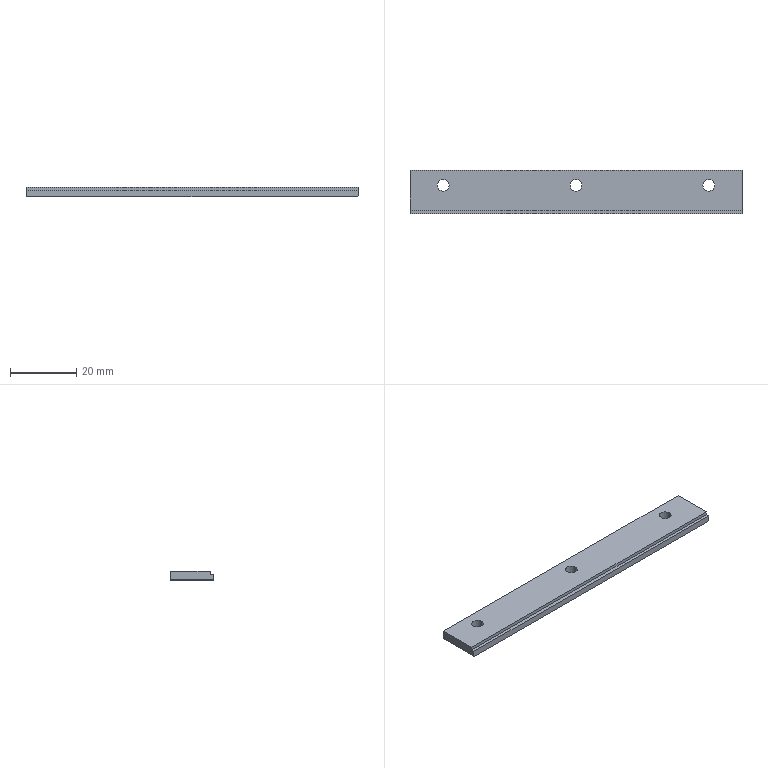Part | STEP file | Feed slide cover_Default | 1 solid | 16 faces | box 100 x 13 x 3 mm | volume 3712 mm3 | plane 10 | cylinder 6 | commonest cylinder face diameters 3.5 x6
STEP:
#1=CARTESIAN_POINT('',(0.,0.,0.));
#2=DIRECTION('',(0.,0.,1.));
#3=DIRECTION('',(1.,0.,0.));
#4=AXIS2_PLACEMENT_3D('',#1,#2,#3);
#5=CARTESIAN_POINT('',(12.886,5.77,0.));
#6=VERTEX_POINT('',#5);
#7=CARTESIAN_POINT('',(12.886,5.77,3.));
#8=VERTEX_POINT('',#7);
#9=CARTESIAN_POINT('',(12.886,5.77,0.));
#10=DIRECTION('',(0.,0.,1.));
#11=VECTOR('',#10,1.);
#12=LINE('',#9,#11);
#13=CARTESIAN_POINT('',(11.136,5.77,0.));
#14=DIRECTION('',(0.,0.,1.));
#15=DIRECTION('',(1.,0.,0.));
#16=AXIS2_PLACEMENT_3D('',#13,#14,#15);
#17=CYLINDRICAL_SURFACE('',#16,1.75);
#18=CARTESIAN_POINT('',(6.283,0.));
#19=DIRECTION('',(0.,1.));
#20=VECTOR('',#19,1.);
#21=LINE('',#18,#20);
#22=(GEOMETRIC_REPRESENTATION_CONTEXT(2)PARAMETRIC_REPRESENTATION_CONTEXT()REPRESENTATION_CONTEXT('',''));
#23=DEFINITIONAL_REPRESENTATION('',(#21),#22);
#24=PCURVE('',#17,#23);
#25=CARTESIAN_POINT('',(11.136,5.77,0.));
#26=DIRECTION('',(0.,0.,1.));
#27=DIRECTION('',(1.,0.,0.));
#28=AXIS2_PLACEMENT_3D('',#25,#26,#27);
#29=CYLINDRICAL_SURFACE('',#28,1.75);
#30=CARTESIAN_POINT('',(0.,0.));
#31=DIRECTION('',(0.,1.));
#32=VECTOR('',#31,1.);
#33=LINE('',#30,#32);
#34=(GEOMETRIC_REPRESENTATION_CONTEXT(2)PARAMETRIC_REPRESENTATION_CONTEXT()REPRESENTATION_CONTEXT('',''));
#35=DEFINITIONAL_REPRESENTATION('',(#33),#34);
#36=PCURVE('',#29,#35);
#37=SURFACE_CURVE('',#12,(#24,#36),.PCURVE_S1.);
#38=EDGE_CURVE('',#6,#8,#37,.T.);
#39=ORIENTED_EDGE('',*,*,#38,.T.);
#40=CARTESIAN_POINT('',(9.386,5.77,3.));
#41=VERTEX_POINT('',#40);
#42=CARTESIAN_POINT('',(11.136,5.77,3.));
#43=DIRECTION('',(0.,0.,1.));
#44=DIRECTION('',(1.,0.,0.));
#45=AXIS2_PLACEMENT_3D('',#42,#43,#44);
#46=CIRCLE('',#45,1.75);
#47=CARTESIAN_POINT('',(0.,3.));
#48=DIRECTION('',(1.,0.));
#49=VECTOR('',#48,1.);
#50=LINE('',#47,#49);
#51=(GEOMETRIC_REPRESENTATION_CONTEXT(2)PARAMETRIC_REPRESENTATION_CONTEXT()REPRESENTATION_CONTEXT('',''));
#52=DEFINITIONAL_REPRESENTATION('',(#50),#51);
#53=PCURVE('',#17,#52);
#54=CARTESIAN_POINT('',(1.136,10.27,3.));
#55=DIRECTION('',(0.,0.,-1.));
#56=DIRECTION('',(-1.,0.,0.));
#57=AXIS2_PLACEMENT_3D('',#54,#55,#56);
#58=PLANE('',#57);
#59=CARTESIAN_POINT('',(-11.75,-4.5));
#60=CARTESIAN_POINT('',(-11.75,-1.469));
#61=CARTESIAN_POINT('',(-9.125,-2.984));
#62=CARTESIAN_POINT('',(-6.5,-4.5));
#63=CARTESIAN_POINT('',(-9.125,-6.016));
#64=CARTESIAN_POINT('',(-11.75,-7.531));
#65=CARTESIAN_POINT('',(-11.75,-4.5));
#66=(BOUNDED_CURVE()B_SPLINE_CURVE(2,(#59,#60,#61,#62,#63,#64,#65),.UNSPECIFIED.,.T.,.F.)B_SPLINE_CURVE_WITH_KNOTS((1,2,2,2,2,1),(-2.094,0.,2.094,4.189,6.283,8.378),.UNSPECIFIED.)CURVE()GEOMETRIC_REPRESENTATION_ITEM()RATIONAL_B_SPLINE_CURVE((1.,0.5,1.,0.5,1.,0.5,1.))REPRESENTATION_ITEM(''));
#67=(GEOMETRIC_REPRESENTATION_CONTEXT(2)PARAMETRIC_REPRESENTATION_CONTEXT()REPRESENTATION_CONTEXT('',''));
#68=DEFINITIONAL_REPRESENTATION('',(#66),#67);
#69=PCURVE('',#58,#68);
#70=SURFACE_CURVE('',#46,(#53,#69),.PCURVE_S1.);
#71=EDGE_CURVE('',#41,#8,#70,.T.);
#72=ORIENTED_EDGE('',*,*,#71,.F.);
#73=CARTESIAN_POINT('',(9.386,5.77,0.));
#74=VERTEX_POINT('',#73);
#75=CARTESIAN_POINT('',(9.386,5.77,0.));
#76=DIRECTION('',(0.,0.,1.));
#77=VECTOR('',#76,1.);
#78=LINE('',#75,#77);
#79=CARTESIAN_POINT('',(3.142,0.));
#80=DIRECTION('',(0.,1.));
#81=VECTOR('',#80,1.);
#82=LINE('',#79,#81);
#83=(GEOMETRIC_REPRESENTATION_CONTEXT(2)PARAMETRIC_REPRESENTATION_CONTEXT()REPRESENTATION_CONTEXT('',''));
#84=DEFINITIONAL_REPRESENTATION('',(#82),#83);
#85=PCURVE('',#17,#84);
#86=CARTESIAN_POINT('',(3.142,0.));
#87=DIRECTION('',(0.,1.));
#88=VECTOR('',#87,1.);
#89=LINE('',#86,#88);
#90=(GEOMETRIC_REPRESENTATION_CONTEXT(2)PARAMETRIC_REPRESENTATION_CONTEXT()REPRESENTATION_CONTEXT('',''));
#91=DEFINITIONAL_REPRESENTATION('',(#89),#90);
#92=PCURVE('',#29,#91);
#93=SURFACE_CURVE('',#78,(#85,#92),.PCURVE_S1.);
#94=EDGE_CURVE('',#74,#41,#93,.T.);
#95=ORIENTED_EDGE('',*,*,#94,.F.);
#96=CARTESIAN_POINT('',(11.136,5.77,0.));
#97=DIRECTION('',(0.,0.,1.));
#98=DIRECTION('',(1.,0.,0.));
#99=AXIS2_PLACEMENT_3D('',#96,#97,#98);
#100=CIRCLE('',#99,1.75);
#101=CARTESIAN_POINT('',(0.,0.));
#102=DIRECTION('',(1.,0.));
#103=VECTOR('',#102,1.);
#104=LINE('',#101,#103);
#105=(GEOMETRIC_REPRESENTATION_CONTEXT(2)PARAMETRIC_REPRESENTATION_CONTEXT()REPRESENTATION_CONTEXT('',''));
#106=DEFINITIONAL_REPRESENTATION('',(#104),#105);
#107=PCURVE('',#17,#106);
#108=CARTESIAN_POINT('',(1.136,10.27,0.));
#109=DIRECTION('',(0.,0.,-1.));
#110=DIRECTION('',(-1.,0.,0.));
#111=AXIS2_PLACEMENT_3D('',#108,#109,#110);
#112=PLANE('',#111);
#113=CARTESIAN_POINT('',(-11.75,-4.5));
#114=CARTESIAN_POINT('',(-11.75,-1.469));
#115=CARTESIAN_POINT('',(-9.125,-2.984));
#116=CARTESIAN_POINT('',(-6.5,-4.5));
#117=CARTESIAN_POINT('',(-9.125,-6.016));
#118=CARTESIAN_POINT('',(-11.75,-7.531));
#119=CARTESIAN_POINT('',(-11.75,-4.5));
#120=(BOUNDED_CURVE()B_SPLINE_CURVE(2,(#113,#114,#115,#116,#117,#118,#119),.UNSPECIFIED.,.T.,.F.)B_SPLINE_CURVE_WITH_KNOTS((1,2,2,2,2,1),(-2.094,0.,2.094,4.189,6.283,8.378),.UNSPECIFIED.)CURVE()GEOMETRIC_REPRESENTATION_ITEM()RATIONAL_B_SPLINE_CURVE((1.,0.5,1.,0.5,1.,0.5,1.))REPRESENTATION_ITEM(''));
#121=(GEOMETRIC_REPRESENTATION_CONTEXT(2)PARAMETRIC_REPRESENTATION_CONTEXT()REPRESENTATION_CONTEXT('',''));
#122=DEFINITIONAL_REPRESENTATION('',(#120),#121);
#123=PCURVE('',#112,#122);
#124=SURFACE_CURVE('',#100,(#107,#123),.PCURVE_S1.);
#125=EDGE_CURVE('',#74,#6,#124,.T.);
#126=ORIENTED_EDGE('',*,*,#125,.T.);
#127=EDGE_LOOP('',(#39,#72,#95,#126));
#128=FACE_BOUND('',#127,.F.);
#129=ADVANCED_FACE('',(#128),#17,.F.);
#130=CARTESIAN_POINT('',(52.886,5.77,0.));
#131=VERTEX_POINT('',#130);
#132=CARTESIAN_POINT('',(52.886,5.77,3.));
#133=VERTEX_POINT('',#132);
#134=CARTESIAN_POINT('',(52.886,5.77,0.));
#135=DIRECTION('',(0.,0.,1.));
#136=VECTOR('',#135,1.);
#137=LINE('',#134,#136);
#138=CARTESIAN_POINT('',(51.136,5.77,0.));
#139=DIRECTION('',(0.,0.,1.));
#140=DIRECTION('',(1.,0.,0.));
#141=AXIS2_PLACEMENT_3D('',#138,#139,#140);
#142=CYLINDRICAL_SURFACE('',#141,1.75);
#143=CARTESIAN_POINT('',(6.283,0.));
#144=DIRECTION('',(0.,1.));
#145=VECTOR('',#144,1.);
#146=LINE('',#143,#145);
#147=(GEOMETRIC_REPRESENTATION_CONTEXT(2)PARAMETRIC_REPRESENTATION_CONTEXT()REPRESENTATION_CONTEXT('',''));
#148=DEFINITIONAL_REPRESENTATION('',(#146),#147);
#149=PCURVE('',#142,#148);
#150=CARTESIAN_POINT('',(51.136,5.77,0.));
#151=DIRECTION('',(0.,0.,1.));
#152=DIRECTION('',(1.,0.,0.));
#153=AXIS2_PLACEMENT_3D('',#150,#151,#152);
#154=CYLINDRICAL_SURFACE('',#153,1.75);
#155=CARTESIAN_POINT('',(0.,0.));
#156=DIRECTION('',(0.,1.));
#157=VECTOR('',#156,1.);
#158=LINE('',#155,#157);
#159=(GEOMETRIC_REPRESENTATION_CONTEXT(2)PARAMETRIC_REPRESENTATION_CONTEXT()REPRESENTATION_CONTEXT('',''));
#160=DEFINITIONAL_REPRESENTATION('',(#158),#159);
#161=PCURVE('',#154,#160);
#162=SURFACE_CURVE('',#137,(#149,#161),.PCURVE_S1.);
#163=EDGE_CURVE('',#131,#133,#162,.T.);
#164=ORIENTED_EDGE('',*,*,#163,.T.);
#165=CARTESIAN_POINT('',(49.386,5.77,3.));
#166=VERTEX_POINT('',#165);
#167=CARTESIAN_POINT('',(51.136,5.77,3.));
#168=DIRECTION('',(0.,0.,1.));
#169=DIRECTION('',(1.,0.,0.));
#170=AXIS2_PLACEMENT_3D('',#167,#168,#169);
#171=CIRCLE('',#170,1.75);
#172=CARTESIAN_POINT('',(0.,3.));
#173=DIRECTION('',(1.,0.));
#174=VECTOR('',#173,1.);
#175=LINE('',#172,#174);
#176=(GEOMETRIC_REPRESENTATION_CONTEXT(2)PARAMETRIC_REPRESENTATION_CONTEXT()REPRESENTATION_CONTEXT('',''));
#177=DEFINITIONAL_REPRESENTATION('',(#175),#176);
#178=PCURVE('',#142,#177);
#179=CARTESIAN_POINT('',(-51.75,-4.5));
#180=CARTESIAN_POINT('',(-51.75,-1.469));
#181=CARTESIAN_POINT('',(-49.125,-2.984));
#182=CARTESIAN_POINT('',(-46.5,-4.5));
#183=CARTESIAN_POINT('',(-49.125,-6.016));
#184=CARTESIAN_POINT('',(-51.75,-7.531));
#185=CARTESIAN_POINT('',(-51.75,-4.5));
#186=(BOUNDED_CURVE()B_SPLINE_CURVE(2,(#179,#180,#181,#182,#183,#184,#185),.UNSPECIFIED.,.T.,.F.)B_SPLINE_CURVE_WITH_KNOTS((1,2,2,2,2,1),(-2.094,0.,2.094,4.189,6.283,8.378),.UNSPECIFIED.)CURVE()GEOMETRIC_REPRESENTATION_ITEM()RATIONAL_B_SPLINE_CURVE((1.,0.5,1.,0.5,1.,0.5,1.))REPRESENTATION_ITEM(''));
#187=(GEOMETRIC_REPRESENTATION_CONTEXT(2)PARAMETRIC_REPRESENTATION_CONTEXT()REPRESENTATION_CONTEXT('',''));
#188=DEFINITIONAL_REPRESENTATION('',(#186),#187);
#189=PCURVE('',#58,#188);
#190=SURFACE_CURVE('',#171,(#178,#189),.PCURVE_S1.);
#191=EDGE_CURVE('',#166,#133,#190,.T.);
#192=ORIENTED_EDGE('',*,*,#191,.F.);
#193=CARTESIAN_POINT('',(49.386,5.77,0.));
#194=VERTEX_POINT('',#193);
#195=CARTESIAN_POINT('',(49.386,5.77,0.));
#196=DIRECTION('',(0.,0.,1.));
#197=VECTOR('',#196,1.);
#198=LINE('',#195,#197);
#199=CARTESIAN_POINT('',(3.142,0.));
#200=DIRECTION('',(0.,1.));
#201=VECTOR('',#200,1.);
#202=LINE('',#199,#201);
#203=(GEOMETRIC_REPRESENTATION_CONTEXT(2)PARAMETRIC_REPRESENTATION_CONTEXT()REPRESENTATION_CONTEXT('',''));
#204=DEFINITIONAL_REPRESENTATION('',(#202),#203);
#205=PCURVE('',#142,#204);
#206=CARTESIAN_POINT('',(3.142,0.));
#207=DIRECTION('',(0.,1.));
#208=VECTOR('',#207,1.);
#209=LINE('',#206,#208);
#210=(GEOMETRIC_REPRESENTATION_CONTEXT(2)PARAMETRIC_REPRESENTATION_CONTEXT()REPRESENTATION_CONTEXT('',''));
#211=DEFINITIONAL_REPRESENTATION('',(#209),#210);
#212=PCURVE('',#154,#211);
#213=SURFACE_CURVE('',#198,(#205,#212),.PCURVE_S1.);
#214=EDGE_CURVE('',#194,#166,#213,.T.);
#215=ORIENTED_EDGE('',*,*,#214,.F.);
#216=CARTESIAN_POINT('',(51.136,5.77,0.));
#217=DIRECTION('',(0.,0.,1.));
#218=DIRECTION('',(1.,0.,0.));
#219=AXIS2_PLACEMENT_3D('',#216,#217,#218);
#220=CIRCLE('',#219,1.75);
#221=CARTESIAN_POINT('',(0.,0.));
#222=DIRECTION('',(1.,0.));
#223=VECTOR('',#222,1.);
#224=LINE('',#221,#223);
#225=(GEOMETRIC_REPRESENTATION_CONTEXT(2)PARAMETRIC_REPRESENTATION_CONTEXT()REPRESENTATION_CONTEXT('',''));
#226=DEFINITIONAL_REPRESENTATION('',(#224),#225);
#227=PCURVE('',#142,#226);
#228=CARTESIAN_POINT('',(-51.75,-4.5));
#229=CARTESIAN_POINT('',(-51.75,-1.469));
#230=CARTESIAN_POINT('',(-49.125,-2.984));
#231=CARTESIAN_POINT('',(-46.5,-4.5));
#232=CARTESIAN_POINT('',(-49.125,-6.016));
#233=CARTESIAN_POINT('',(-51.75,-7.531));
#234=CARTESIAN_POINT('',(-51.75,-4.5));
#235=(BOUNDED_CURVE()B_SPLINE_CURVE(2,(#228,#229,#230,#231,#232,#233,#234),.UNSPECIFIED.,.T.,.F.)B_SPLINE_CURVE_WITH_KNOTS((1,2,2,2,2,1),(-2.094,0.,2.094,4.189,6.283,8.378),.UNSPECIFIED.)CURVE()GEOMETRIC_REPRESENTATION_ITEM()RATIONAL_B_SPLINE_CURVE((1.,0.5,1.,0.5,1.,0.5,1.))REPRESENTATION_ITEM(''));
#236=(GEOMETRIC_REPRESENTATION_CONTEXT(2)PARAMETRIC_REPRESENTATION_CONTEXT()REPRESENTATION_CONTEXT('',''));
#237=DEFINITIONAL_REPRESENTATION('',(#235),#236);
#238=PCURVE('',#112,#237);
#239=SURFACE_CURVE('',#220,(#227,#238),.PCURVE_S1.);
#240=EDGE_CURVE('',#194,#131,#239,.T.);
#241=ORIENTED_EDGE('',*,*,#240,.T.);
#242=EDGE_LOOP('',(#164,#192,#215,#241));
#243=FACE_BOUND('',#242,.F.);
#244=ADVANCED_FACE('',(#243),#142,.F.);
#245=CARTESIAN_POINT('',(92.886,5.77,0.));
#246=VERTEX_POINT('',#245);
#247=CARTESIAN_POINT('',(92.886,5.77,3.));
#248=VERTEX_POINT('',#247);
#249=CARTESIAN_POINT('',(92.886,5.77,0.));
#250=DIRECTION('',(0.,0.,1.));
#251=VECTOR('',#250,1.);
#252=LINE('',#249,#251);
#253=CARTESIAN_POINT('',(91.136,5.77,0.));
#254=DIRECTION('',(0.,0.,1.));
#255=DIRECTION('',(1.,0.,0.));
#256=AXIS2_PLACEMENT_3D('',#253,#254,#255);
#257=CYLINDRICAL_SURFACE('',#256,1.75);
#258=CARTESIAN_POINT('',(6.283,0.));
#259=DIRECTION('',(0.,1.));
#260=VECTOR('',#259,1.);
#261=LINE('',#258,#260);
#262=(GEOMETRIC_REPRESENTATION_CONTEXT(2)PARAMETRIC_REPRESENTATION_CONTEXT()REPRESENTATION_CONTEXT('',''));
#263=DEFINITIONAL_REPRESENTATION('',(#261),#262);
#264=PCURVE('',#257,#263);
#265=CARTESIAN_POINT('',(91.136,5.77,0.));
#266=DIRECTION('',(0.,0.,1.));
#267=DIRECTION('',(1.,0.,0.));
#268=AXIS2_PLACEMENT_3D('',#265,#266,#267);
#269=CYLINDRICAL_SURFACE('',#268,1.75);
#270=CARTESIAN_POINT('',(0.,0.));
#271=DIRECTION('',(0.,1.));
#272=VECTOR('',#271,1.);
#273=LINE('',#270,#272);
#274=(GEOMETRIC_REPRESENTATION_CONTEXT(2)PARAMETRIC_REPRESENTATION_CONTEXT()REPRESENTATION_CONTEXT('',''));
#275=DEFINITIONAL_REPRESENTATION('',(#273),#274);
#276=PCURVE('',#269,#275);
#277=SURFACE_CURVE('',#252,(#264,#276),.PCURVE_S1.);
#278=EDGE_CURVE('',#246,#248,#277,.T.);
#279=ORIENTED_EDGE('',*,*,#278,.T.);
#280=CARTESIAN_POINT('',(89.386,5.77,3.));
#281=VERTEX_POINT('',#280);
#282=CARTESIAN_POINT('',(91.136,5.77,3.));
#283=DIRECTION('',(0.,0.,1.));
#284=DIRECTION('',(1.,0.,0.));
#285=AXIS2_PLACEMENT_3D('',#282,#283,#284);
#286=CIRCLE('',#285,1.75);
#287=CARTESIAN_POINT('',(0.,3.));
#288=DIRECTION('',(1.,0.));
#289=VECTOR('',#288,1.);
#290=LINE('',#287,#289);
#291=(GEOMETRIC_REPRESENTATION_CONTEXT(2)PARAMETRIC_REPRESENTATION_CONTEXT()REPRESENTATION_CONTEXT('',''));
#292=DEFINITIONAL_REPRESENTATION('',(#290),#291);
#293=PCURVE('',#257,#292);
#294=CARTESIAN_POINT('',(-91.75,-4.5));
#295=CARTESIAN_POINT('',(-91.75,-1.469));
#296=CARTESIAN_POINT('',(-89.125,-2.984));
#297=CARTESIAN_POINT('',(-86.5,-4.5));
#298=CARTESIAN_POINT('',(-89.125,-6.016));
#299=CARTESIAN_POINT('',(-91.75,-7.531));
#300=CARTESIAN_POINT('',(-91.75,-4.5));
#301=(BOUNDED_CURVE()B_SPLINE_CURVE(2,(#294,#295,#296,#297,#298,#299,#300),.UNSPECIFIED.,.T.,.F.)B_SPLINE_CURVE_WITH_KNOTS((1,2,2,2,2,1),(-2.094,0.,2.094,4.189,6.283,8.378),.UNSPECIFIED.)CURVE()GEOMETRIC_REPRESENTATION_ITEM()RATIONAL_B_SPLINE_CURVE((1.,0.5,1.,0.5,1.,0.5,1.))REPRESENTATION_ITEM(''));
#302=(GEOMETRIC_REPRESENTATION_CONTEXT(2)PARAMETRIC_REPRESENTATION_CONTEXT()REPRESENTATION_CONTEXT('',''));
#303=DEFINITIONAL_REPRESENTATION('',(#301),#302);
#304=PCURVE('',#58,#303);
#305=SURFACE_CURVE('',#286,(#293,#304),.PCURVE_S1.);
#306=EDGE_CURVE('',#281,#248,#305,.T.);
#307=ORIENTED_EDGE('',*,*,#306,.F.);
#308=CARTESIAN_POINT('',(89.386,5.77,0.));
#309=VERTEX_POINT('',#308);
#310=CARTESIAN_POINT('',(89.386,5.77,0.));
#311=DIRECTION('',(0.,0.,1.));
#312=VECTOR('',#311,1.);
#313=LINE('',#310,#312);
#314=CARTESIAN_POINT('',(3.142,0.));
#315=DIRECTION('',(0.,1.));
#316=VECTOR('',#315,1.);
#317=LINE('',#314,#316);
#318=(GEOMETRIC_REPRESENTATION_CONTEXT(2)PARAMETRIC_REPRESENTATION_CONTEXT()REPRESENTATION_CONTEXT('',''));
#319=DEFINITIONAL_REPRESENTATION('',(#317),#318);
#320=PCURVE('',#257,#319);
#321=CARTESIAN_POINT('',(3.142,0.));
#322=DIRECTION('',(0.,1.));
#323=VECTOR('',#322,1.);
#324=LINE('',#321,#323);
#325=(GEOMETRIC_REPRESENTATION_CONTEXT(2)PARAMETRIC_REPRESENTATION_CONTEXT()REPRESENTATION_CONTEXT('',''));
#326=DEFINITIONAL_REPRESENTATION('',(#324),#325);
#327=PCURVE('',#269,#326);
#328=SURFACE_CURVE('',#313,(#320,#327),.PCURVE_S1.);
#329=EDGE_CURVE('',#309,#281,#328,.T.);
#330=ORIENTED_EDGE('',*,*,#329,.F.);
#331=CARTESIAN_POINT('',(91.136,5.77,0.));
#332=DIRECTION('',(0.,0.,1.));
#333=DIRECTION('',(1.,0.,0.));
#334=AXIS2_PLACEMENT_3D('',#331,#332,#333);
#335=CIRCLE('',#334,1.75);
#336=CARTESIAN_POINT('',(0.,0.));
#337=DIRECTION('',(1.,0.));
#338=VECTOR('',#337,1.);
#339=LINE('',#336,#338);
#340=(GEOMETRIC_REPRESENTATION_CONTEXT(2)PARAMETRIC_REPRESENTATION_CONTEXT()REPRESENTATION_CONTEXT('',''));
#341=DEFINITIONAL_REPRESENTATION('',(#339),#340);
#342=PCURVE('',#257,#341);
#343=CARTESIAN_POINT('',(-91.75,-4.5));
#344=CARTESIAN_POINT('',(-91.75,-1.469));
#345=CARTESIAN_POINT('',(-89.125,-2.984));
#346=CARTESIAN_POINT('',(-86.5,-4.5));
#347=CARTESIAN_POINT('',(-89.125,-6.016));
#348=CARTESIAN_POINT('',(-91.75,-7.531));
#349=CARTESIAN_POINT('',(-91.75,-4.5));
#350=(BOUNDED_CURVE()B_SPLINE_CURVE(2,(#343,#344,#345,#346,#347,#348,#349),.UNSPECIFIED.,.T.,.F.)B_SPLINE_CURVE_WITH_KNOTS((1,2,2,2,2,1),(-2.094,0.,2.094,4.189,6.283,8.378),.UNSPECIFIED.)CURVE()GEOMETRIC_REPRESENTATION_ITEM()RATIONAL_B_SPLINE_CURVE((1.,0.5,1.,0.5,1.,0.5,1.))REPRESENTATION_ITEM(''));
#351=(GEOMETRIC_REPRESENTATION_CONTEXT(2)PARAMETRIC_REPRESENTATION_CONTEXT()REPRESENTATION_CONTEXT('',''));
#352=DEFINITIONAL_REPRESENTATION('',(#350),#351);
#353=PCURVE('',#112,#352);
#354=SURFACE_CURVE('',#335,(#342,#353),.PCURVE_S1.);
#355=EDGE_CURVE('',#309,#246,#354,.T.);
#356=ORIENTED_EDGE('',*,*,#355,.T.);
#357=EDGE_LOOP('',(#279,#307,#330,#356));
#358=FACE_BOUND('',#357,.F.);
#359=ADVANCED_FACE('',(#358),#257,.F.);
#360=CARTESIAN_POINT('',(1.136,10.27,3.));
#361=VERTEX_POINT('',#360);
#362=CARTESIAN_POINT('',(1.136,10.27,0.3));
#363=VERTEX_POINT('',#362);
#364=CARTESIAN_POINT('',(1.136,10.27,3.));
#365=DIRECTION('',(0.,0.,-1.));
#366=VECTOR('',#365,1.);
#367=LINE('',#364,#366);
#368=CARTESIAN_POINT('',(1.136,-2.73,3.));
#369=DIRECTION('',(1.,0.,0.));
#370=DIRECTION('',(0.,0.,-1.));
#371=AXIS2_PLACEMENT_3D('',#368,#369,#370);
#372=PLANE('',#371);
#373=CARTESIAN_POINT('',(0.,13.));
#374=DIRECTION('',(1.,0.));
#375=VECTOR('',#374,1.);
#376=LINE('',#373,#375);
#377=(GEOMETRIC_REPRESENTATION_CONTEXT(2)PARAMETRIC_REPRESENTATION_CONTEXT()REPRESENTATION_CONTEXT('',''));
#378=DEFINITIONAL_REPRESENTATION('',(#376),#377);
#379=PCURVE('',#372,#378);
#380=CARTESIAN_POINT('',(1.136,10.27,3.));
#381=DIRECTION('',(0.,-1.,0.));
#382=DIRECTION('',(0.,0.,-1.));
#383=AXIS2_PLACEMENT_3D('',#380,#381,#382);
#384=PLANE('',#383);
#385=CARTESIAN_POINT('',(0.,0.));
#386=DIRECTION('',(1.,0.));
#387=VECTOR('',#386,1.);
#388=LINE('',#385,#387);
#389=(GEOMETRIC_REPRESENTATION_CONTEXT(2)PARAMETRIC_REPRESENTATION_CONTEXT()REPRESENTATION_CONTEXT('',''));
#390=DEFINITIONAL_REPRESENTATION('',(#388),#389);
#391=PCURVE('',#384,#390);
#392=SURFACE_CURVE('',#367,(#379,#391),.PCURVE_S1.);
#393=EDGE_CURVE('',#361,#363,#392,.T.);
#394=ORIENTED_EDGE('',*,*,#393,.T.);
#395=CARTESIAN_POINT('',(1.136,-2.73,0.3));
#396=VERTEX_POINT('',#395);
#397=CARTESIAN_POINT('',(1.136,-2.73,0.3));
#398=DIRECTION('',(0.,-1.,0.));
#399=VECTOR('',#398,1.);
#400=LINE('',#397,#399);
#401=CARTESIAN_POINT('',(2.7,0.));
#402=DIRECTION('',(0.,-1.));
#403=VECTOR('',#402,1.);
#404=LINE('',#401,#403);
#405=(GEOMETRIC_REPRESENTATION_CONTEXT(2)PARAMETRIC_REPRESENTATION_CONTEXT()REPRESENTATION_CONTEXT('',''));
#406=DEFINITIONAL_REPRESENTATION('',(#404),#405);
#407=PCURVE('',#372,#406);
#408=CARTESIAN_POINT('',(1.136,-2.73,0.3));
#409=DIRECTION('',(-0.7071,0.,-0.7071));
#410=DIRECTION('',(-0.7071,0.,0.7071));
#411=AXIS2_PLACEMENT_3D('',#408,#409,#410);
#412=PLANE('',#411);
#413=CARTESIAN_POINT('',(0.,0.));
#414=DIRECTION('',(0.,-1.));
#415=VECTOR('',#414,1.);
#416=LINE('',#413,#415);
#417=(GEOMETRIC_REPRESENTATION_CONTEXT(2)PARAMETRIC_REPRESENTATION_CONTEXT()REPRESENTATION_CONTEXT('',''));
#418=DEFINITIONAL_REPRESENTATION('',(#416),#417);
#419=PCURVE('',#412,#418);
#420=SURFACE_CURVE('',#400,(#407,#419),.PCURVE_S1.);
#421=EDGE_CURVE('',#363,#396,#420,.T.);
#422=ORIENTED_EDGE('',*,*,#421,.T.);
#423=CARTESIAN_POINT('',(1.136,-2.73,2.));
#424=VERTEX_POINT('',#423);
#425=CARTESIAN_POINT('',(1.136,-2.73,3.));
#426=DIRECTION('',(0.,0.,-1.));
#427=VECTOR('',#426,1.);
#428=LINE('',#425,#427);
#429=CARTESIAN_POINT('',(0.,0.));
#430=DIRECTION('',(1.,0.));
#431=VECTOR('',#430,1.);
#432=LINE('',#429,#431);
#433=(GEOMETRIC_REPRESENTATION_CONTEXT(2)PARAMETRIC_REPRESENTATION_CONTEXT()REPRESENTATION_CONTEXT('',''));
#434=DEFINITIONAL_REPRESENTATION('',(#432),#433);
#435=PCURVE('',#372,#434);
#436=CARTESIAN_POINT('',(1.136,-2.73,3.));
#437=DIRECTION('',(0.,1.,0.));
#438=DIRECTION('',(0.,0.,1.));
#439=AXIS2_PLACEMENT_3D('',#436,#437,#438);
#440=PLANE('',#439);
#441=CARTESIAN_POINT('',(0.,0.));
#442=DIRECTION('',(-1.,0.));
#443=VECTOR('',#442,1.);
#444=LINE('',#441,#443);
#445=(GEOMETRIC_REPRESENTATION_CONTEXT(2)PARAMETRIC_REPRESENTATION_CONTEXT()REPRESENTATION_CONTEXT('',''));
#446=DEFINITIONAL_REPRESENTATION('',(#444),#445);
#447=PCURVE('',#440,#446);
#448=SURFACE_CURVE('',#428,(#435,#447),.PCURVE_S1.);
#449=EDGE_CURVE('',#424,#396,#448,.T.);
#450=ORIENTED_EDGE('',*,*,#449,.F.);
#451=CARTESIAN_POINT('',(1.136,-1.73,2.));
#452=VERTEX_POINT('',#451);
#453=CARTESIAN_POINT('',(1.136,-2.73,2.));
#454=DIRECTION('',(0.,1.,0.));
#455=VECTOR('',#454,1.);
#456=LINE('',#453,#455);
#457=CARTESIAN_POINT('',(1.,0.));
#458=DIRECTION('',(0.,1.));
#459=VECTOR('',#458,1.);
#460=LINE('',#457,#459);
#461=(GEOMETRIC_REPRESENTATION_CONTEXT(2)PARAMETRIC_REPRESENTATION_CONTEXT()REPRESENTATION_CONTEXT('',''));
#462=DEFINITIONAL_REPRESENTATION('',(#460),#461);
#463=PCURVE('',#372,#462);
#464=CARTESIAN_POINT('',(-17.346,-1.73,2.));
#465=DIRECTION('',(0.,0.,-1.));
#466=DIRECTION('',(-1.,0.,0.));
#467=AXIS2_PLACEMENT_3D('',#464,#465,#466);
#468=PLANE('',#467);
#469=CARTESIAN_POINT('',(-18.481,-1.));
#470=DIRECTION('',(0.,1.));
#471=VECTOR('',#470,1.);
#472=LINE('',#469,#471);
#473=(GEOMETRIC_REPRESENTATION_CONTEXT(2)PARAMETRIC_REPRESENTATION_CONTEXT()REPRESENTATION_CONTEXT('',''));
#474=DEFINITIONAL_REPRESENTATION('',(#472),#473);
#475=PCURVE('',#468,#474);
#476=SURFACE_CURVE('',#456,(#463,#475),.PCURVE_S1.);
#477=EDGE_CURVE('',#424,#452,#476,.T.);
#478=ORIENTED_EDGE('',*,*,#477,.T.);
#479=CARTESIAN_POINT('',(1.136,-1.73,3.));
#480=VERTEX_POINT('',#479);
#481=CARTESIAN_POINT('',(1.136,-1.73,3.));
#482=DIRECTION('',(0.,0.,1.));
#483=VECTOR('',#482,1.);
#484=LINE('',#481,#483);
#485=CARTESIAN_POINT('',(0.,1.));
#486=DIRECTION('',(-1.,0.));
#487=VECTOR('',#486,1.);
#488=LINE('',#485,#487);
#489=(GEOMETRIC_REPRESENTATION_CONTEXT(2)PARAMETRIC_REPRESENTATION_CONTEXT()REPRESENTATION_CONTEXT('',''));
#490=DEFINITIONAL_REPRESENTATION('',(#488),#489);
#491=PCURVE('',#372,#490);
#492=CARTESIAN_POINT('',(-17.346,-1.73,2.));
#493=DIRECTION('',(0.,1.,0.));
#494=DIRECTION('',(-1.,0.,0.));
#495=AXIS2_PLACEMENT_3D('',#492,#493,#494);
#496=PLANE('',#495);
#497=CARTESIAN_POINT('',(-18.481,1.));
#498=DIRECTION('',(0.,1.));
#499=VECTOR('',#498,1.);
#500=LINE('',#497,#499);
#501=(GEOMETRIC_REPRESENTATION_CONTEXT(2)PARAMETRIC_REPRESENTATION_CONTEXT()REPRESENTATION_CONTEXT('',''));
#502=DEFINITIONAL_REPRESENTATION('',(#500),#501);
#503=PCURVE('',#496,#502);
#504=SURFACE_CURVE('',#484,(#491,#503),.PCURVE_S1.);
#505=EDGE_CURVE('',#452,#480,#504,.T.);
#506=ORIENTED_EDGE('',*,*,#505,.T.);
#507=CARTESIAN_POINT('',(1.136,-2.73,3.));
#508=DIRECTION('',(0.,-1.,0.));
#509=VECTOR('',#508,1.);
#510=LINE('',#507,#509);
#511=CARTESIAN_POINT('',(0.,0.));
#512=DIRECTION('',(0.,-1.));
#513=VECTOR('',#512,1.);
#514=LINE('',#511,#513);
#515=(GEOMETRIC_REPRESENTATION_CONTEXT(2)PARAMETRIC_REPRESENTATION_CONTEXT()REPRESENTATION_CONTEXT('',''));
#516=DEFINITIONAL_REPRESENTATION('',(#514),#515);
#517=PCURVE('',#372,#516);
#518=CARTESIAN_POINT('',(0.,-13.));
#519=DIRECTION('',(0.,-1.));
#520=VECTOR('',#519,1.);
#521=LINE('',#518,#520);
#522=(GEOMETRIC_REPRESENTATION_CONTEXT(2)PARAMETRIC_REPRESENTATION_CONTEXT()REPRESENTATION_CONTEXT('',''));
#523=DEFINITIONAL_REPRESENTATION('',(#521),#522);
#524=PCURVE('',#58,#523);
#525=SURFACE_CURVE('',#510,(#517,#524),.PCURVE_S1.);
#526=EDGE_CURVE('',#361,#480,#525,.T.);
#527=ORIENTED_EDGE('',*,*,#526,.F.);
#528=EDGE_LOOP('',(#394,#422,#450,#478,#506,#527));
#529=FACE_BOUND('',#528,.T.);
#530=ADVANCED_FACE('',(#529),#372,.F.);
#531=ORIENTED_EDGE('',*,*,#449,.T.);
#532=CARTESIAN_POINT('',(1.436,-2.73,0.));
#533=VERTEX_POINT('',#532);
#534=CARTESIAN_POINT('',(1.136,-2.73,0.3));
#535=DIRECTION('',(0.7071,0.,-0.7071));
#536=VECTOR('',#535,1.);
#537=LINE('',#534,#536);
#538=CARTESIAN_POINT('',(-2.7,0.));
#539=DIRECTION('',(-0.7071,0.7071));
#540=VECTOR('',#539,1.);
#541=LINE('',#538,#540);
#542=(GEOMETRIC_REPRESENTATION_CONTEXT(2)PARAMETRIC_REPRESENTATION_CONTEXT()REPRESENTATION_CONTEXT('',''));
#543=DEFINITIONAL_REPRESENTATION('',(#541),#542);
#544=PCURVE('',#440,#543);
#545=CARTESIAN_POINT('',(0.,0.));
#546=DIRECTION('',(-1.,0.));
#547=VECTOR('',#546,1.);
#548=LINE('',#545,#547);
#549=(GEOMETRIC_REPRESENTATION_CONTEXT(2)PARAMETRIC_REPRESENTATION_CONTEXT()REPRESENTATION_CONTEXT('',''));
#550=DEFINITIONAL_REPRESENTATION('',(#548),#549);
#551=PCURVE('',#412,#550);
#552=SURFACE_CURVE('',#537,(#544,#551),.PCURVE_S1.);
#553=EDGE_CURVE('',#396,#533,#552,.T.);
#554=ORIENTED_EDGE('',*,*,#553,.T.);
#555=CARTESIAN_POINT('',(100.836,-2.73,0.));
#556=VERTEX_POINT('',#555);
#557=CARTESIAN_POINT('',(1.136,-2.73,0.));
#558=DIRECTION('',(1.,0.,0.));
#559=VECTOR('',#558,1.);
#560=LINE('',#557,#559);
#561=CARTESIAN_POINT('',(-3.,0.));
#562=DIRECTION('',(0.,1.));
#563=VECTOR('',#562,1.);
#564=LINE('',#561,#563);
#565=(GEOMETRIC_REPRESENTATION_CONTEXT(2)PARAMETRIC_REPRESENTATION_CONTEXT()REPRESENTATION_CONTEXT('',''));
#566=DEFINITIONAL_REPRESENTATION('',(#564),#565);
#567=PCURVE('',#440,#566);
#568=CARTESIAN_POINT('',(0.,-13.));
#569=DIRECTION('',(-1.,0.));
#570=VECTOR('',#569,1.);
#571=LINE('',#568,#570);
#572=(GEOMETRIC_REPRESENTATION_CONTEXT(2)PARAMETRIC_REPRESENTATION_CONTEXT()REPRESENTATION_CONTEXT('',''));
#573=DEFINITIONAL_REPRESENTATION('',(#571),#572);
#574=PCURVE('',#112,#573);
#575=SURFACE_CURVE('',#560,(#567,#574),.PCURVE_S1.);
#576=EDGE_CURVE('',#533,#556,#575,.T.);
#577=ORIENTED_EDGE('',*,*,#576,.T.);
#578=CARTESIAN_POINT('',(101.136,-2.73,0.3));
#579=VERTEX_POINT('',#578);
#580=CARTESIAN_POINT('',(101.136,-2.73,0.3));
#581=DIRECTION('',(0.7071,0.,0.7071));
#582=VECTOR('',#581,1.);
#583=LINE('',#580,#582);
#584=CARTESIAN_POINT('',(-2.7,100.));
#585=DIRECTION('',(0.7071,0.7071));
#586=VECTOR('',#585,1.);
#587=LINE('',#584,#586);
#588=(GEOMETRIC_REPRESENTATION_CONTEXT(2)PARAMETRIC_REPRESENTATION_CONTEXT()REPRESENTATION_CONTEXT('',''));
#589=DEFINITIONAL_REPRESENTATION('',(#587),#588);
#590=PCURVE('',#440,#589);
#591=CARTESIAN_POINT('',(101.136,-2.73,0.3));
#592=DIRECTION('',(0.7071,0.,-0.7071));
#593=DIRECTION('',(-0.7071,0.,-0.7071));
#594=AXIS2_PLACEMENT_3D('',#591,#592,#593);
#595=PLANE('',#594);
#596=CARTESIAN_POINT('',(0.,0.));
#597=DIRECTION('',(-1.,0.));
#598=VECTOR('',#597,1.);
#599=LINE('',#596,#598);
#600=(GEOMETRIC_REPRESENTATION_CONTEXT(2)PARAMETRIC_REPRESENTATION_CONTEXT()REPRESENTATION_CONTEXT('',''));
#601=DEFINITIONAL_REPRESENTATION('',(#599),#600);
#602=PCURVE('',#595,#601);
#603=SURFACE_CURVE('',#583,(#590,#602),.PCURVE_S1.);
#604=EDGE_CURVE('',#556,#579,#603,.T.);
#605=ORIENTED_EDGE('',*,*,#604,.T.);
#606=CARTESIAN_POINT('',(101.136,-2.73,2.));
#607=VERTEX_POINT('',#606);
#608=CARTESIAN_POINT('',(101.136,-2.73,3.));
#609=DIRECTION('',(0.,0.,-1.));
#610=VECTOR('',#609,1.);
#611=LINE('',#608,#610);
#612=CARTESIAN_POINT('',(0.,100.));
#613=DIRECTION('',(-1.,0.));
#614=VECTOR('',#613,1.);
#615=LINE('',#612,#614);
#616=(GEOMETRIC_REPRESENTATION_CONTEXT(2)PARAMETRIC_REPRESENTATION_CONTEXT()REPRESENTATION_CONTEXT('',''));
#617=DEFINITIONAL_REPRESENTATION('',(#615),#616);
#618=PCURVE('',#440,#617);
#619=CARTESIAN_POINT('',(101.136,-2.73,3.));
#620=DIRECTION('',(-1.,0.,0.));
#621=DIRECTION('',(0.,0.,1.));
#622=AXIS2_PLACEMENT_3D('',#619,#620,#621);
#623=PLANE('',#622);
#624=CARTESIAN_POINT('',(0.,0.));
#625=DIRECTION('',(-1.,0.));
#626=VECTOR('',#625,1.);
#627=LINE('',#624,#626);
#628=(GEOMETRIC_REPRESENTATION_CONTEXT(2)PARAMETRIC_REPRESENTATION_CONTEXT()REPRESENTATION_CONTEXT('',''));
#629=DEFINITIONAL_REPRESENTATION('',(#627),#628);
#630=PCURVE('',#623,#629);
#631=SURFACE_CURVE('',#611,(#618,#630),.PCURVE_S1.);
#632=EDGE_CURVE('',#607,#579,#631,.T.);
#633=ORIENTED_EDGE('',*,*,#632,.F.);
#634=CARTESIAN_POINT('',(1.136,-2.73,2.));
#635=DIRECTION('',(-1.,0.,0.));
#636=VECTOR('',#635,1.);
#637=LINE('',#634,#636);
#638=CARTESIAN_POINT('',(-1.,0.));
#639=DIRECTION('',(0.,-1.));
#640=VECTOR('',#639,1.);
#641=LINE('',#638,#640);
#642=(GEOMETRIC_REPRESENTATION_CONTEXT(2)PARAMETRIC_REPRESENTATION_CONTEXT()REPRESENTATION_CONTEXT('',''));
#643=DEFINITIONAL_REPRESENTATION('',(#641),#642);
#644=PCURVE('',#440,#643);
#645=CARTESIAN_POINT('',(-18.481,-1.));
#646=DIRECTION('',(1.,0.));
#647=VECTOR('',#646,1.);
#648=LINE('',#645,#647);
#649=(GEOMETRIC_REPRESENTATION_CONTEXT(2)PARAMETRIC_REPRESENTATION_CONTEXT()REPRESENTATION_CONTEXT('',''));
#650=DEFINITIONAL_REPRESENTATION('',(#648),#649);
#651=PCURVE('',#468,#650);
#652=SURFACE_CURVE('',#637,(#644,#651),.PCURVE_S1.);
#653=EDGE_CURVE('',#607,#424,#652,.T.);
#654=ORIENTED_EDGE('',*,*,#653,.T.);
#655=EDGE_LOOP('',(#531,#554,#577,#605,#633,#654));
#656=FACE_BOUND('',#655,.T.);
#657=ADVANCED_FACE('',(#656),#440,.F.);
#658=ORIENTED_EDGE('',*,*,#632,.T.);
#659=CARTESIAN_POINT('',(101.136,10.27,0.3));
#660=VERTEX_POINT('',#659);
#661=CARTESIAN_POINT('',(101.136,10.27,0.3));
#662=DIRECTION('',(0.,1.,0.));
#663=VECTOR('',#662,1.);
#664=LINE('',#661,#663);
#665=CARTESIAN_POINT('',(-2.7,13.));
#666=DIRECTION('',(0.,1.));
#667=VECTOR('',#666,1.);
#668=LINE('',#665,#667);
#669=(GEOMETRIC_REPRESENTATION_CONTEXT(2)PARAMETRIC_REPRESENTATION_CONTEXT()REPRESENTATION_CONTEXT('',''));
#670=DEFINITIONAL_REPRESENTATION('',(#668),#669);
#671=PCURVE('',#623,#670);
#672=CARTESIAN_POINT('',(0.,13.));
#673=DIRECTION('',(0.,1.));
#674=VECTOR('',#673,1.);
#675=LINE('',#672,#674);
#676=(GEOMETRIC_REPRESENTATION_CONTEXT(2)PARAMETRIC_REPRESENTATION_CONTEXT()REPRESENTATION_CONTEXT('',''));
#677=DEFINITIONAL_REPRESENTATION('',(#675),#676);
#678=PCURVE('',#595,#677);
#679=SURFACE_CURVE('',#664,(#671,#678),.PCURVE_S1.);
#680=EDGE_CURVE('',#579,#660,#679,.T.);
#681=ORIENTED_EDGE('',*,*,#680,.T.);
#682=CARTESIAN_POINT('',(101.136,10.27,3.));
#683=VERTEX_POINT('',#682);
#684=CARTESIAN_POINT('',(101.136,10.27,3.));
#685=DIRECTION('',(0.,0.,-1.));
#686=VECTOR('',#685,1.);
#687=LINE('',#684,#686);
#688=CARTESIAN_POINT('',(0.,13.));
#689=DIRECTION('',(-1.,0.));
#690=VECTOR('',#689,1.);
#691=LINE('',#688,#690);
#692=(GEOMETRIC_REPRESENTATION_CONTEXT(2)PARAMETRIC_REPRESENTATION_CONTEXT()REPRESENTATION_CONTEXT('',''));
#693=DEFINITIONAL_REPRESENTATION('',(#691),#692);
#694=PCURVE('',#623,#693);
#695=CARTESIAN_POINT('',(0.,100.));
#696=DIRECTION('',(1.,0.));
#697=VECTOR('',#696,1.);
#698=LINE('',#695,#697);
#699=(GEOMETRIC_REPRESENTATION_CONTEXT(2)PARAMETRIC_REPRESENTATION_CONTEXT()REPRESENTATION_CONTEXT('',''));
#700=DEFINITIONAL_REPRESENTATION('',(#698),#699);
#701=PCURVE('',#384,#700);
#702=SURFACE_CURVE('',#687,(#694,#701),.PCURVE_S1.);
#703=EDGE_CURVE('',#683,#660,#702,.T.);
#704=ORIENTED_EDGE('',*,*,#703,.F.);
#705=CARTESIAN_POINT('',(101.136,-1.73,3.));
#706=VERTEX_POINT('',#705);
#707=CARTESIAN_POINT('',(101.136,-2.73,3.));
#708=DIRECTION('',(0.,1.,0.));
#709=VECTOR('',#708,1.);
#710=LINE('',#707,#709);
#711=CARTESIAN_POINT('',(0.,0.));
#712=DIRECTION('',(0.,1.));
#713=VECTOR('',#712,1.);
#714=LINE('',#711,#713);
#715=(GEOMETRIC_REPRESENTATION_CONTEXT(2)PARAMETRIC_REPRESENTATION_CONTEXT()REPRESENTATION_CONTEXT('',''));
#716=DEFINITIONAL_REPRESENTATION('',(#714),#715);
#717=PCURVE('',#623,#716);
#718=CARTESIAN_POINT('',(-100.,-13.));
#719=DIRECTION('',(0.,1.));
#720=VECTOR('',#719,1.);
#721=LINE('',#718,#720);
#722=(GEOMETRIC_REPRESENTATION_CONTEXT(2)PARAMETRIC_REPRESENTATION_CONTEXT()REPRESENTATION_CONTEXT('',''));
#723=DEFINITIONAL_REPRESENTATION('',(#721),#722);
#724=PCURVE('',#58,#723);
#725=SURFACE_CURVE('',#710,(#717,#724),.PCURVE_S1.);
#726=EDGE_CURVE('',#706,#683,#725,.T.);
#727=ORIENTED_EDGE('',*,*,#726,.F.);
#728=CARTESIAN_POINT('',(101.136,-1.73,2.));
#729=VERTEX_POINT('',#728);
#730=CARTESIAN_POINT('',(101.136,-1.73,3.));
#731=DIRECTION('',(0.,0.,-1.));
#732=VECTOR('',#731,1.);
#733=LINE('',#730,#732);
#734=CARTESIAN_POINT('',(0.,1.));
#735=DIRECTION('',(-1.,0.));
#736=VECTOR('',#735,1.);
#737=LINE('',#734,#736);
#738=(GEOMETRIC_REPRESENTATION_CONTEXT(2)PARAMETRIC_REPRESENTATION_CONTEXT()REPRESENTATION_CONTEXT('',''));
#739=DEFINITIONAL_REPRESENTATION('',(#737),#738);
#740=PCURVE('',#623,#739);
#741=CARTESIAN_POINT('',(-118.481,1.));
#742=DIRECTION('',(0.,-1.));
#743=VECTOR('',#742,1.);
#744=LINE('',#741,#743);
#745=(GEOMETRIC_REPRESENTATION_CONTEXT(2)PARAMETRIC_REPRESENTATION_CONTEXT()REPRESENTATION_CONTEXT('',''));
#746=DEFINITIONAL_REPRESENTATION('',(#744),#745);
#747=PCURVE('',#496,#746);
#748=SURFACE_CURVE('',#733,(#740,#747),.PCURVE_S1.);
#749=EDGE_CURVE('',#706,#729,#748,.T.);
#750=ORIENTED_EDGE('',*,*,#749,.T.);
#751=CARTESIAN_POINT('',(101.136,-2.73,2.));
#752=DIRECTION('',(0.,-1.,0.));
#753=VECTOR('',#752,1.);
#754=LINE('',#751,#753);
#755=CARTESIAN_POINT('',(-1.,0.));
#756=DIRECTION('',(0.,-1.));
#757=VECTOR('',#756,1.);
#758=LINE('',#755,#757);
#759=(GEOMETRIC_REPRESENTATION_CONTEXT(2)PARAMETRIC_REPRESENTATION_CONTEXT()REPRESENTATION_CONTEXT('',''));
#760=DEFINITIONAL_REPRESENTATION('',(#758),#759);
#761=PCURVE('',#623,#760);
#762=CARTESIAN_POINT('',(-118.481,-1.));
#763=DIRECTION('',(0.,-1.));
#764=VECTOR('',#763,1.);
#765=LINE('',#762,#764);
#766=(GEOMETRIC_REPRESENTATION_CONTEXT(2)PARAMETRIC_REPRESENTATION_CONTEXT()REPRESENTATION_CONTEXT('',''));
#767=DEFINITIONAL_REPRESENTATION('',(#765),#766);
#768=PCURVE('',#468,#767);
#769=SURFACE_CURVE('',#754,(#761,#768),.PCURVE_S1.);
#770=EDGE_CURVE('',#729,#607,#769,.T.);
#771=ORIENTED_EDGE('',*,*,#770,.T.);
#772=EDGE_LOOP('',(#658,#681,#704,#727,#750,#771));
#773=FACE_BOUND('',#772,.T.);
#774=ADVANCED_FACE('',(#773),#623,.F.);
#775=CARTESIAN_POINT('',(100.836,10.27,0.));
#776=VERTEX_POINT('',#775);
#777=CARTESIAN_POINT('',(1.436,10.27,0.));
#778=VERTEX_POINT('',#777);
#779=CARTESIAN_POINT('',(1.136,10.27,0.));
#780=DIRECTION('',(-1.,0.,0.));
#781=VECTOR('',#780,1.);
#782=LINE('',#779,#781);
#783=CARTESIAN_POINT('',(3.,0.));
#784=DIRECTION('',(0.,-1.));
#785=VECTOR('',#784,1.);
#786=LINE('',#783,#785);
#787=(GEOMETRIC_REPRESENTATION_CONTEXT(2)PARAMETRIC_REPRESENTATION_CONTEXT()REPRESENTATION_CONTEXT('',''));
#788=DEFINITIONAL_REPRESENTATION('',(#786),#787);
#789=PCURVE('',#384,#788);
#790=CARTESIAN_POINT('',(0.,0.));
#791=DIRECTION('',(1.,0.));
#792=VECTOR('',#791,1.);
#793=LINE('',#790,#792);
#794=(GEOMETRIC_REPRESENTATION_CONTEXT(2)PARAMETRIC_REPRESENTATION_CONTEXT()REPRESENTATION_CONTEXT('',''));
#795=DEFINITIONAL_REPRESENTATION('',(#793),#794);
#796=PCURVE('',#112,#795);
#797=SURFACE_CURVE('',#782,(#789,#796),.PCURVE_S1.);
#798=EDGE_CURVE('',#776,#778,#797,.T.);
#799=ORIENTED_EDGE('',*,*,#798,.T.);
#800=CARTESIAN_POINT('',(1.136,10.27,0.3));
#801=DIRECTION('',(-0.7071,0.,0.7071));
#802=VECTOR('',#801,1.);
#803=LINE('',#800,#802);
#804=CARTESIAN_POINT('',(2.7,0.));
#805=DIRECTION('',(-0.7071,-0.7071));
#806=VECTOR('',#805,1.);
#807=LINE('',#804,#806);
#808=(GEOMETRIC_REPRESENTATION_CONTEXT(2)PARAMETRIC_REPRESENTATION_CONTEXT()REPRESENTATION_CONTEXT('',''));
#809=DEFINITIONAL_REPRESENTATION('',(#807),#808);
#810=PCURVE('',#384,#809);
#811=CARTESIAN_POINT('',(0.,13.));
#812=DIRECTION('',(1.,0.));
#813=VECTOR('',#812,1.);
#814=LINE('',#811,#813);
#815=(GEOMETRIC_REPRESENTATION_CONTEXT(2)PARAMETRIC_REPRESENTATION_CONTEXT()REPRESENTATION_CONTEXT('',''));
#816=DEFINITIONAL_REPRESENTATION('',(#814),#815);
#817=PCURVE('',#412,#816);
#818=SURFACE_CURVE('',#803,(#810,#817),.PCURVE_S1.);
#819=EDGE_CURVE('',#778,#363,#818,.T.);
#820=ORIENTED_EDGE('',*,*,#819,.T.);
#821=ORIENTED_EDGE('',*,*,#393,.F.);
#822=CARTESIAN_POINT('',(1.136,10.27,3.));
#823=DIRECTION('',(-1.,0.,0.));
#824=VECTOR('',#823,1.);
#825=LINE('',#822,#824);
#826=CARTESIAN_POINT('',(0.,0.));
#827=DIRECTION('',(0.,-1.));
#828=VECTOR('',#827,1.);
#829=LINE('',#826,#828);
#830=(GEOMETRIC_REPRESENTATION_CONTEXT(2)PARAMETRIC_REPRESENTATION_CONTEXT()REPRESENTATION_CONTEXT('',''));
#831=DEFINITIONAL_REPRESENTATION('',(#829),#830);
#832=PCURVE('',#384,#831);
#833=CARTESIAN_POINT('',(0.,0.));
#834=DIRECTION('',(1.,0.));
#835=VECTOR('',#834,1.);
#836=LINE('',#833,#835);
#837=(GEOMETRIC_REPRESENTATION_CONTEXT(2)PARAMETRIC_REPRESENTATION_CONTEXT()REPRESENTATION_CONTEXT('',''));
#838=DEFINITIONAL_REPRESENTATION('',(#836),#837);
#839=PCURVE('',#58,#838);
#840=SURFACE_CURVE('',#825,(#832,#839),.PCURVE_S1.);
#841=EDGE_CURVE('',#683,#361,#840,.T.);
#842=ORIENTED_EDGE('',*,*,#841,.F.);
#843=ORIENTED_EDGE('',*,*,#703,.T.);
#844=CARTESIAN_POINT('',(101.136,10.27,0.3));
#845=DIRECTION('',(-0.7071,0.,-0.7071));
#846=VECTOR('',#845,1.);
#847=LINE('',#844,#846);
#848=CARTESIAN_POINT('',(2.7,100.));
#849=DIRECTION('',(0.7071,-0.7071));
#850=VECTOR('',#849,1.);
#851=LINE('',#848,#850);
#852=(GEOMETRIC_REPRESENTATION_CONTEXT(2)PARAMETRIC_REPRESENTATION_CONTEXT()REPRESENTATION_CONTEXT('',''));
#853=DEFINITIONAL_REPRESENTATION('',(#851),#852);
#854=PCURVE('',#384,#853);
#855=CARTESIAN_POINT('',(0.,13.));
#856=DIRECTION('',(1.,0.));
#857=VECTOR('',#856,1.);
#858=LINE('',#855,#857);
#859=(GEOMETRIC_REPRESENTATION_CONTEXT(2)PARAMETRIC_REPRESENTATION_CONTEXT()REPRESENTATION_CONTEXT('',''));
#860=DEFINITIONAL_REPRESENTATION('',(#858),#859);
#861=PCURVE('',#595,#860);
#862=SURFACE_CURVE('',#847,(#854,#861),.PCURVE_S1.);
#863=EDGE_CURVE('',#660,#776,#862,.T.);
#864=ORIENTED_EDGE('',*,*,#863,.T.);
#865=EDGE_LOOP('',(#799,#820,#821,#842,#843,#864));
#866=FACE_BOUND('',#865,.T.);
#867=ADVANCED_FACE('',(#866),#384,.F.);
#868=CARTESIAN_POINT('',(51.136,5.77,3.));
#869=DIRECTION('',(0.,0.,1.));
#870=DIRECTION('',(1.,0.,0.));
#871=AXIS2_PLACEMENT_3D('',#868,#869,#870);
#872=CIRCLE('',#871,1.75);
#873=CARTESIAN_POINT('',(-51.75,-4.5));
#874=CARTESIAN_POINT('',(-51.75,-1.469));
#875=CARTESIAN_POINT('',(-49.125,-2.984));
#876=CARTESIAN_POINT('',(-46.5,-4.5));
#877=CARTESIAN_POINT('',(-49.125,-6.016));
#878=CARTESIAN_POINT('',(-51.75,-7.531));
#879=CARTESIAN_POINT('',(-51.75,-4.5));
#880=(BOUNDED_CURVE()B_SPLINE_CURVE(2,(#873,#874,#875,#876,#877,#878,#879),.UNSPECIFIED.,.T.,.F.)B_SPLINE_CURVE_WITH_KNOTS((1,2,2,2,2,1),(-2.094,0.,2.094,4.189,6.283,8.378),.UNSPECIFIED.)CURVE()GEOMETRIC_REPRESENTATION_ITEM()RATIONAL_B_SPLINE_CURVE((1.,0.5,1.,0.5,1.,0.5,1.))REPRESENTATION_ITEM(''));
#881=(GEOMETRIC_REPRESENTATION_CONTEXT(2)PARAMETRIC_REPRESENTATION_CONTEXT()REPRESENTATION_CONTEXT('',''));
#882=DEFINITIONAL_REPRESENTATION('',(#880),#881);
#883=PCURVE('',#58,#882);
#884=CARTESIAN_POINT('',(0.,3.));
#885=DIRECTION('',(1.,0.));
#886=VECTOR('',#885,1.);
#887=LINE('',#884,#886);
#888=(GEOMETRIC_REPRESENTATION_CONTEXT(2)PARAMETRIC_REPRESENTATION_CONTEXT()REPRESENTATION_CONTEXT('',''));
#889=DEFINITIONAL_REPRESENTATION('',(#887),#888);
#890=PCURVE('',#154,#889);
#891=SURFACE_CURVE('',#872,(#883,#890),.PCURVE_S1.);
#892=EDGE_CURVE('',#133,#166,#891,.T.);
#893=ORIENTED_EDGE('',*,*,#892,.F.);
#894=ORIENTED_EDGE('',*,*,#191,.F.);
#895=EDGE_LOOP('',(#893,#894));
#896=FACE_BOUND('',#895,.T.);
#897=CARTESIAN_POINT('',(91.136,5.77,3.));
#898=DIRECTION('',(0.,0.,1.));
#899=DIRECTION('',(1.,0.,0.));
#900=AXIS2_PLACEMENT_3D('',#897,#898,#899);
#901=CIRCLE('',#900,1.75);
#902=CARTESIAN_POINT('',(-91.75,-4.5));
#903=CARTESIAN_POINT('',(-91.75,-1.469));
#904=CARTESIAN_POINT('',(-89.125,-2.984));
#905=CARTESIAN_POINT('',(-86.5,-4.5));
#906=CARTESIAN_POINT('',(-89.125,-6.016));
#907=CARTESIAN_POINT('',(-91.75,-7.531));
#908=CARTESIAN_POINT('',(-91.75,-4.5));
#909=(BOUNDED_CURVE()B_SPLINE_CURVE(2,(#902,#903,#904,#905,#906,#907,#908),.UNSPECIFIED.,.T.,.F.)B_SPLINE_CURVE_WITH_KNOTS((1,2,2,2,2,1),(-2.094,0.,2.094,4.189,6.283,8.378),.UNSPECIFIED.)CURVE()GEOMETRIC_REPRESENTATION_ITEM()RATIONAL_B_SPLINE_CURVE((1.,0.5,1.,0.5,1.,0.5,1.))REPRESENTATION_ITEM(''));
#910=(GEOMETRIC_REPRESENTATION_CONTEXT(2)PARAMETRIC_REPRESENTATION_CONTEXT()REPRESENTATION_CONTEXT('',''));
#911=DEFINITIONAL_REPRESENTATION('',(#909),#910);
#912=PCURVE('',#58,#911);
#913=CARTESIAN_POINT('',(0.,3.));
#914=DIRECTION('',(1.,0.));
#915=VECTOR('',#914,1.);
#916=LINE('',#913,#915);
#917=(GEOMETRIC_REPRESENTATION_CONTEXT(2)PARAMETRIC_REPRESENTATION_CONTEXT()REPRESENTATION_CONTEXT('',''));
#918=DEFINITIONAL_REPRESENTATION('',(#916),#917);
#919=PCURVE('',#269,#918);
#920=SURFACE_CURVE('',#901,(#912,#919),.PCURVE_S1.);
#921=EDGE_CURVE('',#248,#281,#920,.T.);
#922=ORIENTED_EDGE('',*,*,#921,.F.);
#923=ORIENTED_EDGE('',*,*,#306,.F.);
#924=EDGE_LOOP('',(#922,#923));
#925=FACE_BOUND('',#924,.T.);
#926=ORIENTED_EDGE('',*,*,#526,.T.);
#927=CARTESIAN_POINT('',(1.136,-1.73,3.));
#928=DIRECTION('',(1.,0.,0.));
#929=VECTOR('',#928,1.);
#930=LINE('',#927,#929);
#931=CARTESIAN_POINT('',(0.,-12.));
#932=DIRECTION('',(-1.,0.));
#933=VECTOR('',#932,1.);
#934=LINE('',#931,#933);
#935=(GEOMETRIC_REPRESENTATION_CONTEXT(2)PARAMETRIC_REPRESENTATION_CONTEXT()REPRESENTATION_CONTEXT('',''));
#936=DEFINITIONAL_REPRESENTATION('',(#934),#935);
#937=PCURVE('',#58,#936);
#938=CARTESIAN_POINT('',(-18.481,1.));
#939=DIRECTION('',(-1.,0.));
#940=VECTOR('',#939,1.);
#941=LINE('',#938,#940);
#942=(GEOMETRIC_REPRESENTATION_CONTEXT(2)PARAMETRIC_REPRESENTATION_CONTEXT()REPRESENTATION_CONTEXT('',''));
#943=DEFINITIONAL_REPRESENTATION('',(#941),#942);
#944=PCURVE('',#496,#943);
#945=SURFACE_CURVE('',#930,(#937,#944),.PCURVE_S1.);
#946=EDGE_CURVE('',#480,#706,#945,.T.);
#947=ORIENTED_EDGE('',*,*,#946,.T.);
#948=ORIENTED_EDGE('',*,*,#726,.T.);
#949=ORIENTED_EDGE('',*,*,#841,.T.);
#950=EDGE_LOOP('',(#926,#947,#948,#949));
#951=FACE_BOUND('',#950,.T.);
#952=CARTESIAN_POINT('',(11.136,5.77,3.));
#953=DIRECTION('',(0.,0.,1.));
#954=DIRECTION('',(1.,0.,0.));
#955=AXIS2_PLACEMENT_3D('',#952,#953,#954);
#956=CIRCLE('',#955,1.75);
#957=CARTESIAN_POINT('',(-11.75,-4.5));
#958=CARTESIAN_POINT('',(-11.75,-1.469));
#959=CARTESIAN_POINT('',(-9.125,-2.984));
#960=CARTESIAN_POINT('',(-6.5,-4.5));
#961=CARTESIAN_POINT('',(-9.125,-6.016));
#962=CARTESIAN_POINT('',(-11.75,-7.531));
#963=CARTESIAN_POINT('',(-11.75,-4.5));
#964=(BOUNDED_CURVE()B_SPLINE_CURVE(2,(#957,#958,#959,#960,#961,#962,#963),.UNSPECIFIED.,.T.,.F.)B_SPLINE_CURVE_WITH_KNOTS((1,2,2,2,2,1),(-2.094,0.,2.094,4.189,6.283,8.378),.UNSPECIFIED.)CURVE()GEOMETRIC_REPRESENTATION_ITEM()RATIONAL_B_SPLINE_CURVE((1.,0.5,1.,0.5,1.,0.5,1.))REPRESENTATION_ITEM(''));
#965=(GEOMETRIC_REPRESENTATION_CONTEXT(2)PARAMETRIC_REPRESENTATION_CONTEXT()REPRESENTATION_CONTEXT('',''));
#966=DEFINITIONAL_REPRESENTATION('',(#964),#965);
#967=PCURVE('',#58,#966);
#968=CARTESIAN_POINT('',(0.,3.));
#969=DIRECTION('',(1.,0.));
#970=VECTOR('',#969,1.);
#971=LINE('',#968,#970);
#972=(GEOMETRIC_REPRESENTATION_CONTEXT(2)PARAMETRIC_REPRESENTATION_CONTEXT()REPRESENTATION_CONTEXT('',''));
#973=DEFINITIONAL_REPRESENTATION('',(#971),#972);
#974=PCURVE('',#29,#973);
#975=SURFACE_CURVE('',#956,(#967,#974),.PCURVE_S1.);
#976=EDGE_CURVE('',#8,#41,#975,.T.);
#977=ORIENTED_EDGE('',*,*,#976,.F.);
#978=ORIENTED_EDGE('',*,*,#71,.F.);
#979=EDGE_LOOP('',(#977,#978));
#980=FACE_BOUND('',#979,.T.);
#981=ADVANCED_FACE('',(#896,#925,#951,#980),#58,.F.);
#982=CARTESIAN_POINT('',(51.136,5.77,0.));
#983=DIRECTION('',(0.,0.,1.));
#984=DIRECTION('',(1.,0.,0.));
#985=AXIS2_PLACEMENT_3D('',#982,#983,#984);
#986=CIRCLE('',#985,1.75);
#987=CARTESIAN_POINT('',(-51.75,-4.5));
#988=CARTESIAN_POINT('',(-51.75,-1.469));
#989=CARTESIAN_POINT('',(-49.125,-2.984));
#990=CARTESIAN_POINT('',(-46.5,-4.5));
#991=CARTESIAN_POINT('',(-49.125,-6.016));
#992=CARTESIAN_POINT('',(-51.75,-7.531));
#993=CARTESIAN_POINT('',(-51.75,-4.5));
#994=(BOUNDED_CURVE()B_SPLINE_CURVE(2,(#987,#988,#989,#990,#991,#992,#993),.UNSPECIFIED.,.T.,.F.)B_SPLINE_CURVE_WITH_KNOTS((1,2,2,2,2,1),(-2.094,0.,2.094,4.189,6.283,8.378),.UNSPECIFIED.)CURVE()GEOMETRIC_REPRESENTATION_ITEM()RATIONAL_B_SPLINE_CURVE((1.,0.5,1.,0.5,1.,0.5,1.))REPRESENTATION_ITEM(''));
#995=(GEOMETRIC_REPRESENTATION_CONTEXT(2)PARAMETRIC_REPRESENTATION_CONTEXT()REPRESENTATION_CONTEXT('',''));
#996=DEFINITIONAL_REPRESENTATION('',(#994),#995);
#997=PCURVE('',#112,#996);
#998=CARTESIAN_POINT('',(0.,0.));
#999=DIRECTION('',(1.,0.));
#1000=VECTOR('',#999,1.);
#1001=LINE('',#998,#1000);
#1002=(GEOMETRIC_REPRESENTATION_CONTEXT(2)PARAMETRIC_REPRESENTATION_CONTEXT()REPRESENTATION_CONTEXT('',''));
#1003=DEFINITIONAL_REPRESENTATION('',(#1001),#1002);
#1004=PCURVE('',#154,#1003);
#1005=SURFACE_CURVE('',#986,(#997,#1004),.PCURVE_S1.);
#1006=EDGE_CURVE('',#131,#194,#1005,.T.);
#1007=ORIENTED_EDGE('',*,*,#1006,.T.);
#1008=ORIENTED_EDGE('',*,*,#240,.T.);
#1009=EDGE_LOOP('',(#1007,#1008));
#1010=FACE_BOUND('',#1009,.T.);
#1011=CARTESIAN_POINT('',(91.136,5.77,0.));
#1012=DIRECTION('',(0.,0.,1.));
#1013=DIRECTION('',(1.,0.,0.));
#1014=AXIS2_PLACEMENT_3D('',#1011,#1012,#1013);
#1015=CIRCLE('',#1014,1.75);
#1016=CARTESIAN_POINT('',(-91.75,-4.5));
#1017=CARTESIAN_POINT('',(-91.75,-1.469));
#1018=CARTESIAN_POINT('',(-89.125,-2.984));
#1019=CARTESIAN_POINT('',(-86.5,-4.5));
#1020=CARTESIAN_POINT('',(-89.125,-6.016));
#1021=CARTESIAN_POINT('',(-91.75,-7.531));
#1022=CARTESIAN_POINT('',(-91.75,-4.5));
#1023=(BOUNDED_CURVE()B_SPLINE_CURVE(2,(#1016,#1017,#1018,#1019,#1020,#1021,#1022),.UNSPECIFIED.,.T.,.F.)B_SPLINE_CURVE_WITH_KNOTS((1,2,2,2,2,1),(-2.094,0.,2.094,4.189,6.283,8.378),.UNSPECIFIED.)CURVE()GEOMETRIC_REPRESENTATION_ITEM()RATIONAL_B_SPLINE_CURVE((1.,0.5,1.,0.5,1.,0.5,1.))REPRESENTATION_ITEM(''));
#1024=(GEOMETRIC_REPRESENTATION_CONTEXT(2)PARAMETRIC_REPRESENTATION_CONTEXT()REPRESENTATION_CONTEXT('',''));
#1025=DEFINITIONAL_REPRESENTATION('',(#1023),#1024);
#1026=PCURVE('',#112,#1025);
#1027=CARTESIAN_POINT('',(0.,0.));
#1028=DIRECTION('',(1.,0.));
#1029=VECTOR('',#1028,1.);
#1030=LINE('',#1027,#1029);
#1031=(GEOMETRIC_REPRESENTATION_CONTEXT(2)PARAMETRIC_REPRESENTATION_CONTEXT()REPRESENTATION_CONTEXT('',''));
#1032=DEFINITIONAL_REPRESENTATION('',(#1030),#1031);
#1033=PCURVE('',#269,#1032);
#1034=SURFACE_CURVE('',#1015,(#1026,#1033),.PCURVE_S1.);
#1035=EDGE_CURVE('',#246,#309,#1034,.T.);
#1036=ORIENTED_EDGE('',*,*,#1035,.T.);
#1037=ORIENTED_EDGE('',*,*,#355,.T.);
#1038=EDGE_LOOP('',(#1036,#1037));
#1039=FACE_BOUND('',#1038,.T.);
#1040=ORIENTED_EDGE('',*,*,#576,.F.);
#1041=CARTESIAN_POINT('',(1.436,10.27,0.));
#1042=DIRECTION('',(0.,1.,0.));
#1043=VECTOR('',#1042,1.);
#1044=LINE('',#1041,#1043);
#1045=CARTESIAN_POINT('',(-0.3,0.));
#1046=DIRECTION('',(0.,1.));
#1047=VECTOR('',#1046,1.);
#1048=LINE('',#1045,#1047);
#1049=(GEOMETRIC_REPRESENTATION_CONTEXT(2)PARAMETRIC_REPRESENTATION_CONTEXT()REPRESENTATION_CONTEXT('',''));
#1050=DEFINITIONAL_REPRESENTATION('',(#1048),#1049);
#1051=PCURVE('',#112,#1050);
#1052=CARTESIAN_POINT('',(-0.4243,13.));
#1053=DIRECTION('',(0.,1.));
#1054=VECTOR('',#1053,1.);
#1055=LINE('',#1052,#1054);
#1056=(GEOMETRIC_REPRESENTATION_CONTEXT(2)PARAMETRIC_REPRESENTATION_CONTEXT()REPRESENTATION_CONTEXT('',''));
#1057=DEFINITIONAL_REPRESENTATION('',(#1055),#1056);
#1058=PCURVE('',#412,#1057);
#1059=SURFACE_CURVE('',#1044,(#1051,#1058),.PCURVE_S1.);
#1060=EDGE_CURVE('',#533,#778,#1059,.T.);
#1061=ORIENTED_EDGE('',*,*,#1060,.T.);
#1062=ORIENTED_EDGE('',*,*,#798,.F.);
#1063=CARTESIAN_POINT('',(100.836,-2.73,0.));
#1064=DIRECTION('',(0.,-1.,0.));
#1065=VECTOR('',#1064,1.);
#1066=LINE('',#1063,#1065);
#1067=CARTESIAN_POINT('',(-99.7,-13.));
#1068=DIRECTION('',(0.,-1.));
#1069=VECTOR('',#1068,1.);
#1070=LINE('',#1067,#1069);
#1071=(GEOMETRIC_REPRESENTATION_CONTEXT(2)PARAMETRIC_REPRESENTATION_CONTEXT()REPRESENTATION_CONTEXT('',''));
#1072=DEFINITIONAL_REPRESENTATION('',(#1070),#1071);
#1073=PCURVE('',#112,#1072);
#1074=CARTESIAN_POINT('',(0.4243,0.));
#1075=DIRECTION('',(0.,-1.));
#1076=VECTOR('',#1075,1.);
#1077=LINE('',#1074,#1076);
#1078=(GEOMETRIC_REPRESENTATION_CONTEXT(2)PARAMETRIC_REPRESENTATION_CONTEXT()REPRESENTATION_CONTEXT('',''));
#1079=DEFINITIONAL_REPRESENTATION('',(#1077),#1078);
#1080=PCURVE('',#595,#1079);
#1081=SURFACE_CURVE('',#1066,(#1073,#1080),.PCURVE_S1.);
#1082=EDGE_CURVE('',#776,#556,#1081,.T.);
#1083=ORIENTED_EDGE('',*,*,#1082,.T.);
#1084=EDGE_LOOP('',(#1040,#1061,#1062,#1083));
#1085=FACE_BOUND('',#1084,.T.);
#1086=CARTESIAN_POINT('',(11.136,5.77,0.));
#1087=DIRECTION('',(0.,0.,1.));
#1088=DIRECTION('',(1.,0.,0.));
#1089=AXIS2_PLACEMENT_3D('',#1086,#1087,#1088);
#1090=CIRCLE('',#1089,1.75);
#1091=CARTESIAN_POINT('',(-11.75,-4.5));
#1092=CARTESIAN_POINT('',(-11.75,-1.469));
#1093=CARTESIAN_POINT('',(-9.125,-2.984));
#1094=CARTESIAN_POINT('',(-6.5,-4.5));
#1095=CARTESIAN_POINT('',(-9.125,-6.016));
#1096=CARTESIAN_POINT('',(-11.75,-7.531));
#1097=CARTESIAN_POINT('',(-11.75,-4.5));
#1098=(BOUNDED_CURVE()B_SPLINE_CURVE(2,(#1091,#1092,#1093,#1094,#1095,#1096,#1097),.UNSPECIFIED.,.T.,.F.)B_SPLINE_CURVE_WITH_KNOTS((1,2,2,2,2,1),(-2.094,0.,2.094,4.189,6.283,8.378),.UNSPECIFIED.)CURVE()GEOMETRIC_REPRESENTATION_ITEM()RATIONAL_B_SPLINE_CURVE((1.,0.5,1.,0.5,1.,0.5,1.))REPRESENTATION_ITEM(''));
#1099=(GEOMETRIC_REPRESENTATION_CONTEXT(2)PARAMETRIC_REPRESENTATION_CONTEXT()REPRESENTATION_CONTEXT('',''));
#1100=DEFINITIONAL_REPRESENTATION('',(#1098),#1099);
#1101=PCURVE('',#112,#1100);
#1102=CARTESIAN_POINT('',(0.,0.));
#1103=DIRECTION('',(1.,0.));
#1104=VECTOR('',#1103,1.);
#1105=LINE('',#1102,#1104);
#1106=(GEOMETRIC_REPRESENTATION_CONTEXT(2)PARAMETRIC_REPRESENTATION_CONTEXT()REPRESENTATION_CONTEXT('',''));
#1107=DEFINITIONAL_REPRESENTATION('',(#1105),#1106);
#1108=PCURVE('',#29,#1107);
#1109=SURFACE_CURVE('',#1090,(#1101,#1108),.PCURVE_S1.);
#1110=EDGE_CURVE('',#6,#74,#1109,.T.);
#1111=ORIENTED_EDGE('',*,*,#1110,.T.);
#1112=ORIENTED_EDGE('',*,*,#125,.T.);
#1113=EDGE_LOOP('',(#1111,#1112));
#1114=FACE_BOUND('',#1113,.T.);
#1115=ADVANCED_FACE('',(#1010,#1039,#1085,#1114),#112,.T.);
#1116=ORIENTED_EDGE('',*,*,#653,.F.);
#1117=ORIENTED_EDGE('',*,*,#770,.F.);
#1118=CARTESIAN_POINT('',(-17.346,-1.73,2.));
#1119=DIRECTION('',(-1.,0.,0.));
#1120=VECTOR('',#1119,1.);
#1121=LINE('',#1118,#1120);
#1122=CARTESIAN_POINT('',(0.,0.));
#1123=DIRECTION('',(1.,0.));
#1124=VECTOR('',#1123,1.);
#1125=LINE('',#1122,#1124);
#1126=(GEOMETRIC_REPRESENTATION_CONTEXT(2)PARAMETRIC_REPRESENTATION_CONTEXT()REPRESENTATION_CONTEXT('',''));
#1127=DEFINITIONAL_REPRESENTATION('',(#1125),#1126);
#1128=PCURVE('',#468,#1127);
#1129=CARTESIAN_POINT('',(0.,0.));
#1130=DIRECTION('',(1.,0.));
#1131=VECTOR('',#1130,1.);
#1132=LINE('',#1129,#1131);
#1133=(GEOMETRIC_REPRESENTATION_CONTEXT(2)PARAMETRIC_REPRESENTATION_CONTEXT()REPRESENTATION_CONTEXT('',''));
#1134=DEFINITIONAL_REPRESENTATION('',(#1132),#1133);
#1135=PCURVE('',#496,#1134);
#1136=SURFACE_CURVE('',#1121,(#1128,#1135),.PCURVE_S1.);
#1137=EDGE_CURVE('',#729,#452,#1136,.T.);
#1138=ORIENTED_EDGE('',*,*,#1137,.T.);
#1139=ORIENTED_EDGE('',*,*,#477,.F.);
#1140=EDGE_LOOP('',(#1116,#1117,#1138,#1139));
#1141=FACE_BOUND('',#1140,.T.);
#1142=ADVANCED_FACE('',(#1141),#468,.F.);
#1143=ORIENTED_EDGE('',*,*,#1137,.F.);
#1144=ORIENTED_EDGE('',*,*,#749,.F.);
#1145=ORIENTED_EDGE('',*,*,#946,.F.);
#1146=ORIENTED_EDGE('',*,*,#505,.F.);
#1147=EDGE_LOOP('',(#1143,#1144,#1145,#1146));
#1148=FACE_BOUND('',#1147,.T.);
#1149=ADVANCED_FACE('',(#1148),#496,.F.);
#1150=ORIENTED_EDGE('',*,*,#819,.F.);
#1151=ORIENTED_EDGE('',*,*,#1060,.F.);
#1152=ORIENTED_EDGE('',*,*,#553,.F.);
#1153=ORIENTED_EDGE('',*,*,#421,.F.);
#1154=EDGE_LOOP('',(#1150,#1151,#1152,#1153));
#1155=FACE_BOUND('',#1154,.T.);
#1156=ADVANCED_FACE('',(#1155),#412,.T.);
#1157=ORIENTED_EDGE('',*,*,#604,.F.);
#1158=ORIENTED_EDGE('',*,*,#1082,.F.);
#1159=ORIENTED_EDGE('',*,*,#863,.F.);
#1160=ORIENTED_EDGE('',*,*,#680,.F.);
#1161=EDGE_LOOP('',(#1157,#1158,#1159,#1160));
#1162=FACE_BOUND('',#1161,.T.);
#1163=ADVANCED_FACE('',(#1162),#595,.T.);
#1164=ORIENTED_EDGE('',*,*,#921,.F.);
#1165=ORIENTED_EDGE('',*,*,#278,.F.);
#1166=ORIENTED_EDGE('',*,*,#1035,.T.);
#1167=ORIENTED_EDGE('',*,*,#329,.T.);
#1168=EDGE_LOOP('',(#1164,#1165,#1166,#1167));
#1169=FACE_BOUND('',#1168,.F.);
#1170=ADVANCED_FACE('',(#1169),#269,.F.);
#1171=ORIENTED_EDGE('',*,*,#892,.F.);
#1172=ORIENTED_EDGE('',*,*,#163,.F.);
#1173=ORIENTED_EDGE('',*,*,#1006,.T.);
#1174=ORIENTED_EDGE('',*,*,#214,.T.);
#1175=EDGE_LOOP('',(#1171,#1172,#1173,#1174));
#1176=FACE_BOUND('',#1175,.F.);
#1177=ADVANCED_FACE('',(#1176),#154,.F.);
#1178=ORIENTED_EDGE('',*,*,#976,.F.);
#1179=ORIENTED_EDGE('',*,*,#38,.F.);
#1180=ORIENTED_EDGE('',*,*,#1110,.T.);
#1181=ORIENTED_EDGE('',*,*,#94,.T.);
#1182=EDGE_LOOP('',(#1178,#1179,#1180,#1181));
#1183=FACE_BOUND('',#1182,.F.);
#1184=ADVANCED_FACE('',(#1183),#29,.F.);
#1185=CLOSED_SHELL('',(#129,#244,#359,#530,#657,#774,#867,#981,#1115,#1142,#1149,#1156,#1163,#1170,#1177,#1184));
#1186=MANIFOLD_SOLID_BREP('',#1185);
#1187=(LENGTH_UNIT()NAMED_UNIT(*)SI_UNIT(.MILLI.,.METRE.));
#1188=UNCERTAINTY_MEASURE_WITH_UNIT(LENGTH_MEASURE(0.0000001),#1187,'','');
#1189=(NAMED_UNIT(*)PLANE_ANGLE_UNIT()SI_UNIT($,.RADIAN.));
#1190=(NAMED_UNIT(*)SI_UNIT($,.STERADIAN.)SOLID_ANGLE_UNIT());
#1191=(GEOMETRIC_REPRESENTATION_CONTEXT(3)GLOBAL_UNCERTAINTY_ASSIGNED_CONTEXT((#1188))GLOBAL_UNIT_ASSIGNED_CONTEXT((#1187,#1189,#1190))REPRESENTATION_CONTEXT('',''));
#1192=ADVANCED_BREP_SHAPE_REPRESENTATION('',(#4,#1186),#1191);